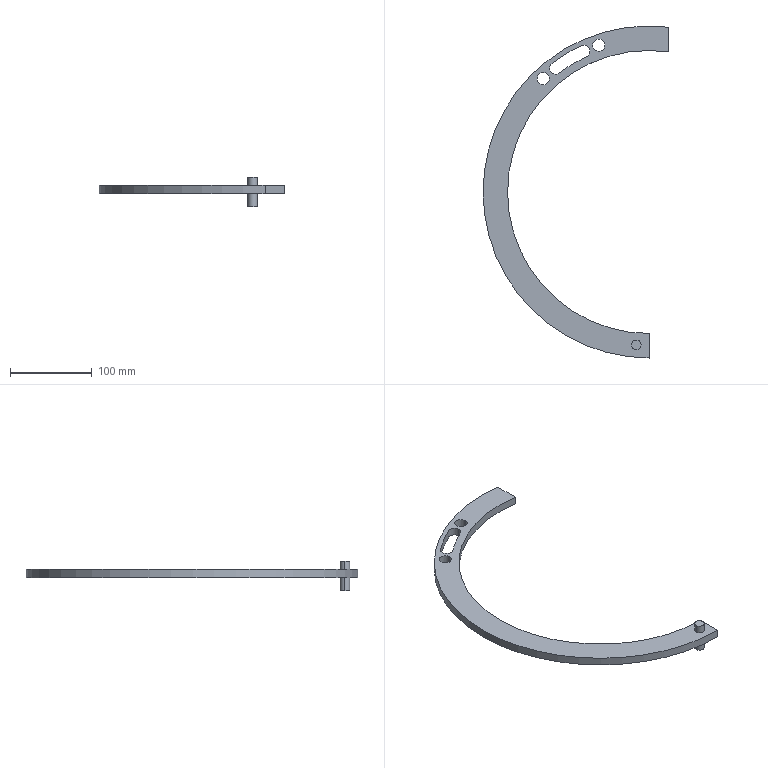Part | SolidWorks | features Cut 1, Extrusion 1, ICE 1 | 1 solid | 21 faces | box 227.579 x 406.59 x 36 mm | volume 176233 mm3 | cylinder 15 | plane 6 | commonest cylinder face diameters 15 x7 11.641 x4 346.59 x1 365 x1 395 x1 406.59 x1
STEP:
#1=CARTESIAN_POINT('',(-413.724,321.633,-10.));
#2=VERTEX_POINT('',#1);
#3=CARTESIAN_POINT('',(-428.724,321.633,-10.));
#4=VERTEX_POINT('',#3);
#5=CARTESIAN_POINT('',(-421.224,321.633,-10.));
#6=DIRECTION('',(0.,0.,-1.));
#7=DIRECTION('',(-1.,0.,0.));
#8=AXIS2_PLACEMENT_3D('',#5,#6,#7);
#9=CIRCLE('',#8,7.5);
#10=EDGE_CURVE('',#2,#4,#9,.T.);
#11=ORIENTED_EDGE('',*,*,#10,.T.);
#12=CARTESIAN_POINT('',(-428.724,321.633,0.));
#13=VERTEX_POINT('',#12);
#14=CARTESIAN_POINT('',(-428.724,321.633,-26.));
#15=DIRECTION('',(0.,0.,1.));
#16=VECTOR('',#15,1000.);
#17=LINE('',#14,#16);
#18=EDGE_CURVE('',#4,#13,#17,.T.);
#19=ORIENTED_EDGE('',*,*,#18,.T.);
#20=CARTESIAN_POINT('',(-413.724,321.633,0.));
#21=VERTEX_POINT('',#20);
#22=CARTESIAN_POINT('',(-421.224,321.633,0.));
#23=DIRECTION('',(0.,0.,-1.));
#24=DIRECTION('',(-1.,0.,0.));
#25=AXIS2_PLACEMENT_3D('',#22,#23,#24);
#26=CIRCLE('',#25,7.5);
#27=EDGE_CURVE('',#21,#13,#26,.T.);
#28=ORIENTED_EDGE('',*,*,#27,.F.);
#29=CARTESIAN_POINT('',(-413.724,321.633,-26.));
#30=DIRECTION('',(0.,0.,1.));
#31=VECTOR('',#30,1000.);
#32=LINE('',#29,#31);
#33=EDGE_CURVE('',#2,#21,#32,.T.);
#34=ORIENTED_EDGE('',*,*,#33,.F.);
#35=EDGE_LOOP('',(#11,#19,#28,#34));
#36=FACE_OUTER_BOUND('',#35,.T.);
#37=CARTESIAN_POINT('',(-421.224,321.633,-26.));
#38=DIRECTION('',(0.,0.,1.));
#39=DIRECTION('',(1.,0.,0.));
#40=AXIS2_PLACEMENT_3D('',#37,#38,#39);
#41=CYLINDRICAL_SURFACE('',#40,7.5);
#42=ADVANCED_FACE('',(#36),#41,.F.);
#43=CARTESIAN_POINT('',(-345.629,362.487,-10.));
#44=VERTEX_POINT('',#43);
#45=CARTESIAN_POINT('',(-360.629,362.487,-10.));
#46=VERTEX_POINT('',#45);
#47=CARTESIAN_POINT('',(-353.129,362.487,-10.));
#48=DIRECTION('',(0.,0.,-1.));
#49=DIRECTION('',(-1.,0.,0.));
#50=AXIS2_PLACEMENT_3D('',#47,#48,#49);
#51=CIRCLE('',#50,7.5);
#52=EDGE_CURVE('',#44,#46,#51,.T.);
#53=ORIENTED_EDGE('',*,*,#52,.T.);
#54=CARTESIAN_POINT('',(-360.629,362.487,0.));
#55=VERTEX_POINT('',#54);
#56=CARTESIAN_POINT('',(-360.629,362.487,-26.));
#57=DIRECTION('',(0.,0.,1.));
#58=VECTOR('',#57,1000.);
#59=LINE('',#56,#58);
#60=EDGE_CURVE('',#46,#55,#59,.T.);
#61=ORIENTED_EDGE('',*,*,#60,.T.);
#62=CARTESIAN_POINT('',(-345.629,362.487,0.));
#63=VERTEX_POINT('',#62);
#64=CARTESIAN_POINT('',(-353.129,362.487,0.));
#65=DIRECTION('',(0.,0.,-1.));
#66=DIRECTION('',(-1.,0.,0.));
#67=AXIS2_PLACEMENT_3D('',#64,#65,#66);
#68=CIRCLE('',#67,7.5);
#69=EDGE_CURVE('',#63,#55,#68,.T.);
#70=ORIENTED_EDGE('',*,*,#69,.F.);
#71=CARTESIAN_POINT('',(-345.629,362.487,-26.));
#72=DIRECTION('',(0.,0.,1.));
#73=VECTOR('',#72,1000.);
#74=LINE('',#71,#73);
#75=EDGE_CURVE('',#44,#63,#74,.T.);
#76=ORIENTED_EDGE('',*,*,#75,.F.);
#77=EDGE_LOOP('',(#53,#61,#70,#76));
#78=FACE_OUTER_BOUND('',#77,.T.);
#79=CARTESIAN_POINT('',(-353.129,362.487,-26.));
#80=DIRECTION('',(0.,0.,1.));
#81=DIRECTION('',(1.,0.,0.));
#82=AXIS2_PLACEMENT_3D('',#79,#80,#81);
#83=CYLINDRICAL_SURFACE('',#82,7.5);
#84=ADVANCED_FACE('',(#78),#83,.F.);
#85=CARTESIAN_POINT('',(-374.845,361.823,-10.));
#86=VERTEX_POINT('',#85);
#87=CARTESIAN_POINT('',(-364.183,355.022,-10.));
#88=VERTEX_POINT('',#87);
#89=CARTESIAN_POINT('',(-371.683,355.022,-10.));
#90=DIRECTION('',(0.,0.,-1.));
#91=DIRECTION('',(-1.,0.,0.));
#92=AXIS2_PLACEMENT_3D('',#89,#90,#91);
#93=CIRCLE('',#92,7.5);
#94=EDGE_CURVE('',#86,#88,#93,.T.);
#95=ORIENTED_EDGE('',*,*,#94,.T.);
#96=CARTESIAN_POINT('',(-364.183,355.022,0.));
#97=VERTEX_POINT('',#96);
#98=CARTESIAN_POINT('',(-364.183,355.022,-26.));
#99=DIRECTION('',(0.,0.,1.));
#100=VECTOR('',#99,1000.);
#101=LINE('',#98,#100);
#102=EDGE_CURVE('',#88,#97,#101,.T.);
#103=ORIENTED_EDGE('',*,*,#102,.T.);
#104=CARTESIAN_POINT('',(-374.845,361.823,0.));
#105=VERTEX_POINT('',#104);
#106=CARTESIAN_POINT('',(-371.683,355.022,0.));
#107=DIRECTION('',(0.,0.,-1.));
#108=DIRECTION('',(-1.,0.,0.));
#109=AXIS2_PLACEMENT_3D('',#106,#107,#108);
#110=CIRCLE('',#109,7.5);
#111=EDGE_CURVE('',#105,#97,#110,.T.);
#112=ORIENTED_EDGE('',*,*,#111,.F.);
#113=CARTESIAN_POINT('',(-374.845,361.823,-26.));
#114=DIRECTION('',(0.,0.,1.));
#115=VECTOR('',#114,1000.);
#116=LINE('',#113,#115);
#117=EDGE_CURVE('',#86,#105,#116,.T.);
#118=ORIENTED_EDGE('',*,*,#117,.F.);
#119=EDGE_LOOP('',(#95,#103,#112,#118));
#120=FACE_OUTER_BOUND('',#119,.T.);
#121=CARTESIAN_POINT('',(-371.683,355.022,-26.));
#122=DIRECTION('',(0.,0.,1.));
#123=DIRECTION('',(1.,0.,0.));
#124=AXIS2_PLACEMENT_3D('',#121,#122,#123);
#125=CYLINDRICAL_SURFACE('',#124,7.5);
#126=ADVANCED_FACE('',(#120),#125,.F.);
#127=CARTESIAN_POINT('',(-301.381,-4.52,-26.));
#128=VERTEX_POINT('',#127);
#129=CARTESIAN_POINT('',(-313.022,-4.52,-26.));
#130=VERTEX_POINT('',#129);
#131=CARTESIAN_POINT('',(-307.202,-4.52,-26.));
#132=DIRECTION('',(0.,0.,1.));
#133=DIRECTION('',(1.,0.,0.));
#134=AXIS2_PLACEMENT_3D('',#131,#132,#133);
#135=CIRCLE('',#134,5.82);
#136=EDGE_CURVE('',#128,#130,#135,.T.);
#137=ORIENTED_EDGE('',*,*,#136,.T.);
#138=CARTESIAN_POINT('',(-313.022,-4.52,-10.));
#139=VERTEX_POINT('',#138);
#140=CARTESIAN_POINT('',(-313.022,-4.52,-26.));
#141=DIRECTION('',(0.,0.,1.));
#142=VECTOR('',#141,1000.);
#143=LINE('',#140,#142);
#144=EDGE_CURVE('',#130,#139,#143,.T.);
#145=ORIENTED_EDGE('',*,*,#144,.T.);
#146=CARTESIAN_POINT('',(-301.381,-4.52,-10.));
#147=VERTEX_POINT('',#146);
#148=CARTESIAN_POINT('',(-307.202,-4.52,-10.));
#149=DIRECTION('',(0.,0.,-1.));
#150=DIRECTION('',(-1.,0.,0.));
#151=AXIS2_PLACEMENT_3D('',#148,#149,#150);
#152=CIRCLE('',#151,5.82);
#153=EDGE_CURVE('',#139,#147,#152,.T.);
#154=ORIENTED_EDGE('',*,*,#153,.T.);
#155=CARTESIAN_POINT('',(-301.381,-4.52,-26.));
#156=DIRECTION('',(0.,0.,1.));
#157=VECTOR('',#156,1000.);
#158=LINE('',#155,#157);
#159=EDGE_CURVE('',#128,#147,#158,.T.);
#160=ORIENTED_EDGE('',*,*,#159,.F.);
#161=EDGE_LOOP('',(#137,#145,#154,#160));
#162=FACE_OUTER_BOUND('',#161,.T.);
#163=CARTESIAN_POINT('',(-307.202,-4.52,-26.));
#164=DIRECTION('',(0.,0.,1.));
#165=DIRECTION('',(1.,0.,0.));
#166=AXIS2_PLACEMENT_3D('',#163,#164,#165);
#167=CYLINDRICAL_SURFACE('',#166,5.82);
#168=ADVANCED_FACE('',(#162),#167,.T.);
#169=CARTESIAN_POINT('',(-313.022,-4.52,0.));
#170=VERTEX_POINT('',#169);
#171=CARTESIAN_POINT('',(-301.381,-4.52,0.));
#172=VERTEX_POINT('',#171);
#173=CARTESIAN_POINT('',(-307.202,-4.52,0.));
#174=DIRECTION('',(0.,0.,-1.));
#175=DIRECTION('',(-1.,0.,0.));
#176=AXIS2_PLACEMENT_3D('',#173,#174,#175);
#177=CIRCLE('',#176,5.82);
#178=EDGE_CURVE('',#170,#172,#177,.T.);
#179=ORIENTED_EDGE('',*,*,#178,.F.);
#180=CARTESIAN_POINT('',(-313.022,-4.52,10.));
#181=VERTEX_POINT('',#180);
#182=CARTESIAN_POINT('',(-313.022,-4.52,-26.));
#183=DIRECTION('',(0.,0.,1.));
#184=VECTOR('',#183,1000.);
#185=LINE('',#182,#184);
#186=EDGE_CURVE('',#170,#181,#185,.T.);
#187=ORIENTED_EDGE('',*,*,#186,.T.);
#188=CARTESIAN_POINT('',(-301.381,-4.52,10.));
#189=VERTEX_POINT('',#188);
#190=CARTESIAN_POINT('',(-307.202,-4.52,10.));
#191=DIRECTION('',(0.,0.,1.));
#192=DIRECTION('',(1.,0.,0.));
#193=AXIS2_PLACEMENT_3D('',#190,#191,#192);
#194=CIRCLE('',#193,5.82);
#195=EDGE_CURVE('',#189,#181,#194,.T.);
#196=ORIENTED_EDGE('',*,*,#195,.F.);
#197=CARTESIAN_POINT('',(-301.381,-4.52,-26.));
#198=DIRECTION('',(0.,0.,1.));
#199=VECTOR('',#198,1000.);
#200=LINE('',#197,#199);
#201=EDGE_CURVE('',#172,#189,#200,.T.);
#202=ORIENTED_EDGE('',*,*,#201,.F.);
#203=EDGE_LOOP('',(#179,#187,#196,#202));
#204=FACE_OUTER_BOUND('',#203,.T.);
#205=CARTESIAN_POINT('',(-307.202,-4.52,-26.));
#206=DIRECTION('',(0.,0.,1.));
#207=DIRECTION('',(1.,0.,0.));
#208=AXIS2_PLACEMENT_3D('',#205,#206,#207);
#209=CYLINDRICAL_SURFACE('',#208,5.82);
#210=ADVANCED_FACE('',(#204),#209,.T.);
#211=ORIENTED_EDGE('',*,*,#10,.F.);
#212=CARTESIAN_POINT('',(-421.224,321.633,-10.));
#213=DIRECTION('',(0.,0.,-1.));
#214=DIRECTION('',(-1.,0.,0.));
#215=AXIS2_PLACEMENT_3D('',#212,#213,#214);
#216=CIRCLE('',#215,7.5);
#217=EDGE_CURVE('',#4,#2,#216,.T.);
#218=ORIENTED_EDGE('',*,*,#217,.F.);
#219=EDGE_LOOP('',(#211,#218));
#220=FACE_BOUND('',#219,.T.);
#221=ORIENTED_EDGE('',*,*,#52,.F.);
#222=CARTESIAN_POINT('',(-353.129,362.487,-10.));
#223=DIRECTION('',(0.,0.,-1.));
#224=DIRECTION('',(-1.,0.,0.));
#225=AXIS2_PLACEMENT_3D('',#222,#223,#224);
#226=CIRCLE('',#225,7.5);
#227=EDGE_CURVE('',#46,#44,#226,.T.);
#228=ORIENTED_EDGE('',*,*,#227,.F.);
#229=EDGE_LOOP('',(#221,#228));
#230=FACE_BOUND('',#229,.T.);
#231=ORIENTED_EDGE('',*,*,#94,.F.);
#232=CARTESIAN_POINT('',(-410.433,340.469,-10.));
#233=VERTEX_POINT('',#232);
#234=CARTESIAN_POINT('',(-291.585,182.731,-10.));
#235=DIRECTION('',(0.,0.,-1.));
#236=DIRECTION('',(-1.,0.,0.));
#237=AXIS2_PLACEMENT_3D('',#234,#235,#236);
#238=CIRCLE('',#237,197.5);
#239=EDGE_CURVE('',#233,#86,#238,.T.);
#240=ORIENTED_EDGE('',*,*,#239,.F.);
#241=CARTESIAN_POINT('',(-401.406,328.489,-10.));
#242=VERTEX_POINT('',#241);
#243=CARTESIAN_POINT('',(-405.919,334.479,-10.));
#244=DIRECTION('',(0.,0.,-1.));
#245=DIRECTION('',(-1.,0.,0.));
#246=AXIS2_PLACEMENT_3D('',#243,#244,#245);
#247=CIRCLE('',#246,7.5);
#248=EDGE_CURVE('',#242,#233,#247,.T.);
#249=ORIENTED_EDGE('',*,*,#248,.F.);
#250=CARTESIAN_POINT('',(-368.522,348.221,-10.));
#251=VERTEX_POINT('',#250);
#252=CARTESIAN_POINT('',(-291.585,182.731,-10.));
#253=DIRECTION('',(0.,0.,1.));
#254=DIRECTION('',(-1.,0.,0.));
#255=AXIS2_PLACEMENT_3D('',#252,#253,#254);
#256=CIRCLE('',#255,182.5);
#257=EDGE_CURVE('',#251,#242,#256,.T.);
#258=ORIENTED_EDGE('',*,*,#257,.F.);
#259=CARTESIAN_POINT('',(-371.683,355.022,-10.));
#260=DIRECTION('',(0.,0.,-1.));
#261=DIRECTION('',(-1.,0.,0.));
#262=AXIS2_PLACEMENT_3D('',#259,#260,#261);
#263=CIRCLE('',#262,7.5);
#264=EDGE_CURVE('',#88,#251,#263,.T.);
#265=ORIENTED_EDGE('',*,*,#264,.F.);
#266=EDGE_LOOP('',(#231,#240,#249,#258,#265));
#267=FACE_BOUND('',#266,.T.);
#268=CARTESIAN_POINT('',(-307.202,-4.52,-10.));
#269=DIRECTION('',(0.,0.,-1.));
#270=DIRECTION('',(-1.,0.,0.));
#271=AXIS2_PLACEMENT_3D('',#268,#269,#270);
#272=CIRCLE('',#271,5.82);
#273=EDGE_CURVE('',#147,#139,#272,.T.);
#274=ORIENTED_EDGE('',*,*,#273,.F.);
#275=ORIENTED_EDGE('',*,*,#153,.F.);
#276=EDGE_LOOP('',(#274,#275));
#277=FACE_BOUND('',#276,.T.);
#278=CARTESIAN_POINT('',(-291.585,9.436,-10.));
#279=VERTEX_POINT('',#278);
#280=CARTESIAN_POINT('',(-267.302,354.316,-10.));
#281=VERTEX_POINT('',#280);
#282=CARTESIAN_POINT('',(-291.585,182.731,-10.));
#283=DIRECTION('',(0.,0.,-1.));
#284=DIRECTION('',(-1.,0.,0.));
#285=AXIS2_PLACEMENT_3D('',#282,#283,#284);
#286=CIRCLE('',#285,173.295);
#287=EDGE_CURVE('',#279,#281,#286,.T.);
#288=ORIENTED_EDGE('',*,*,#287,.F.);
#289=CARTESIAN_POINT('',(-291.585,-20.564,-10.));
#290=VERTEX_POINT('',#289);
#291=CARTESIAN_POINT('',(-291.585,9.436,-10.));
#292=DIRECTION('',(0.,1.,0.));
#293=VECTOR('',#292,1000.);
#294=LINE('',#291,#293);
#295=EDGE_CURVE('',#290,#279,#294,.T.);
#296=ORIENTED_EDGE('',*,*,#295,.F.);
#297=CARTESIAN_POINT('',(-267.317,384.572,-10.));
#298=VERTEX_POINT('',#297);
#299=CARTESIAN_POINT('',(-291.585,182.731,-10.));
#300=DIRECTION('',(0.,0.,1.));
#301=DIRECTION('',(-1.,0.,0.));
#302=AXIS2_PLACEMENT_3D('',#299,#300,#301);
#303=CIRCLE('',#302,203.295);
#304=EDGE_CURVE('',#298,#290,#303,.T.);
#305=ORIENTED_EDGE('',*,*,#304,.F.);
#306=CARTESIAN_POINT('',(-267.317,384.572,-10.));
#307=DIRECTION('',(-0.0005094,1.,0.));
#308=VECTOR('',#307,1000.);
#309=LINE('',#306,#308);
#310=EDGE_CURVE('',#281,#298,#309,.T.);
#311=ORIENTED_EDGE('',*,*,#310,.F.);
#312=EDGE_LOOP('',(#288,#296,#305,#311));
#313=FACE_OUTER_BOUND('',#312,.T.);
#314=CARTESIAN_POINT('',(-291.585,182.731,-10.));
#315=DIRECTION('',(0.,0.,-1.));
#316=DIRECTION('',(-1.,0.,0.));
#317=AXIS2_PLACEMENT_3D('',#314,#315,#316);
#318=PLANE('',#317);
#319=ADVANCED_FACE('',(#220,#230,#267,#277,#313),#318,.T.);
#320=ORIENTED_EDGE('',*,*,#27,.T.);
#321=CARTESIAN_POINT('',(-421.224,321.633,0.));
#322=DIRECTION('',(0.,0.,-1.));
#323=DIRECTION('',(-1.,0.,0.));
#324=AXIS2_PLACEMENT_3D('',#321,#322,#323);
#325=CIRCLE('',#324,7.5);
#326=EDGE_CURVE('',#13,#21,#325,.T.);
#327=ORIENTED_EDGE('',*,*,#326,.T.);
#328=EDGE_LOOP('',(#320,#327));
#329=FACE_BOUND('',#328,.T.);
#330=ORIENTED_EDGE('',*,*,#69,.T.);
#331=CARTESIAN_POINT('',(-353.129,362.487,0.));
#332=DIRECTION('',(0.,0.,-1.));
#333=DIRECTION('',(-1.,0.,0.));
#334=AXIS2_PLACEMENT_3D('',#331,#332,#333);
#335=CIRCLE('',#334,7.5);
#336=EDGE_CURVE('',#55,#63,#335,.T.);
#337=ORIENTED_EDGE('',*,*,#336,.T.);
#338=EDGE_LOOP('',(#330,#337));
#339=FACE_BOUND('',#338,.T.);
#340=CARTESIAN_POINT('',(-410.433,340.469,0.));
#341=VERTEX_POINT('',#340);
#342=CARTESIAN_POINT('',(-291.585,182.731,0.));
#343=DIRECTION('',(0.,0.,-1.));
#344=DIRECTION('',(-1.,0.,0.));
#345=AXIS2_PLACEMENT_3D('',#342,#343,#344);
#346=CIRCLE('',#345,197.5);
#347=EDGE_CURVE('',#341,#105,#346,.T.);
#348=ORIENTED_EDGE('',*,*,#347,.T.);
#349=ORIENTED_EDGE('',*,*,#111,.T.);
#350=CARTESIAN_POINT('',(-368.522,348.221,0.));
#351=VERTEX_POINT('',#350);
#352=CARTESIAN_POINT('',(-371.683,355.022,0.));
#353=DIRECTION('',(0.,0.,-1.));
#354=DIRECTION('',(-1.,0.,0.));
#355=AXIS2_PLACEMENT_3D('',#352,#353,#354);
#356=CIRCLE('',#355,7.5);
#357=EDGE_CURVE('',#97,#351,#356,.T.);
#358=ORIENTED_EDGE('',*,*,#357,.T.);
#359=CARTESIAN_POINT('',(-401.406,328.489,0.));
#360=VERTEX_POINT('',#359);
#361=CARTESIAN_POINT('',(-291.585,182.731,0.));
#362=DIRECTION('',(0.,0.,1.));
#363=DIRECTION('',(-1.,0.,0.));
#364=AXIS2_PLACEMENT_3D('',#361,#362,#363);
#365=CIRCLE('',#364,182.5);
#366=EDGE_CURVE('',#351,#360,#365,.T.);
#367=ORIENTED_EDGE('',*,*,#366,.T.);
#368=CARTESIAN_POINT('',(-405.919,334.479,0.));
#369=DIRECTION('',(0.,0.,-1.));
#370=DIRECTION('',(-1.,0.,0.));
#371=AXIS2_PLACEMENT_3D('',#368,#369,#370);
#372=CIRCLE('',#371,7.5);
#373=EDGE_CURVE('',#360,#341,#372,.T.);
#374=ORIENTED_EDGE('',*,*,#373,.T.);
#375=EDGE_LOOP('',(#348,#349,#358,#367,#374));
#376=FACE_BOUND('',#375,.T.);
#377=CARTESIAN_POINT('',(-307.202,-4.52,0.));
#378=DIRECTION('',(0.,0.,-1.));
#379=DIRECTION('',(-1.,0.,0.));
#380=AXIS2_PLACEMENT_3D('',#377,#378,#379);
#381=CIRCLE('',#380,5.82);
#382=EDGE_CURVE('',#172,#170,#381,.T.);
#383=ORIENTED_EDGE('',*,*,#382,.T.);
#384=ORIENTED_EDGE('',*,*,#178,.T.);
#385=EDGE_LOOP('',(#383,#384));
#386=FACE_BOUND('',#385,.T.);
#387=CARTESIAN_POINT('',(-291.585,9.436,0.));
#388=VERTEX_POINT('',#387);
#389=CARTESIAN_POINT('',(-267.302,354.316,0.));
#390=VERTEX_POINT('',#389);
#391=CARTESIAN_POINT('',(-291.585,182.731,0.));
#392=DIRECTION('',(0.,0.,-1.));
#393=DIRECTION('',(-1.,0.,0.));
#394=AXIS2_PLACEMENT_3D('',#391,#392,#393);
#395=CIRCLE('',#394,173.295);
#396=EDGE_CURVE('',#388,#390,#395,.T.);
#397=ORIENTED_EDGE('',*,*,#396,.T.);
#398=CARTESIAN_POINT('',(-267.317,384.572,0.));
#399=VERTEX_POINT('',#398);
#400=CARTESIAN_POINT('',(-267.317,384.572,0.));
#401=DIRECTION('',(-0.0005094,1.,0.));
#402=VECTOR('',#401,1000.);
#403=LINE('',#400,#402);
#404=EDGE_CURVE('',#390,#399,#403,.T.);
#405=ORIENTED_EDGE('',*,*,#404,.T.);
#406=CARTESIAN_POINT('',(-291.585,-20.564,0.));
#407=VERTEX_POINT('',#406);
#408=CARTESIAN_POINT('',(-291.585,182.731,0.));
#409=DIRECTION('',(0.,0.,1.));
#410=DIRECTION('',(1.,0.,0.));
#411=AXIS2_PLACEMENT_3D('',#408,#409,#410);
#412=CIRCLE('',#411,203.295);
#413=EDGE_CURVE('',#399,#407,#412,.T.);
#414=ORIENTED_EDGE('',*,*,#413,.T.);
#415=CARTESIAN_POINT('',(-291.585,9.436,0.));
#416=DIRECTION('',(0.,1.,0.));
#417=VECTOR('',#416,1000.);
#418=LINE('',#415,#417);
#419=EDGE_CURVE('',#407,#388,#418,.T.);
#420=ORIENTED_EDGE('',*,*,#419,.T.);
#421=EDGE_LOOP('',(#397,#405,#414,#420));
#422=FACE_OUTER_BOUND('',#421,.T.);
#423=CARTESIAN_POINT('',(-291.585,182.731,0.));
#424=DIRECTION('',(0.,0.,-1.));
#425=DIRECTION('',(-1.,0.,0.));
#426=AXIS2_PLACEMENT_3D('',#423,#424,#425);
#427=PLANE('',#426);
#428=ADVANCED_FACE('',(#329,#339,#376,#386,#422),#427,.F.);
#429=CARTESIAN_POINT('',(-267.302,354.316,-475.948));
#430=DIRECTION('',(0.,0.,1.));
#431=VECTOR('',#430,1000.);
#432=LINE('',#429,#431);
#433=EDGE_CURVE('',#281,#390,#432,.T.);
#434=ORIENTED_EDGE('',*,*,#433,.F.);
#435=ORIENTED_EDGE('',*,*,#310,.T.);
#436=CARTESIAN_POINT('',(-267.317,384.572,-475.948));
#437=DIRECTION('',(0.,0.,1.));
#438=VECTOR('',#437,1000.);
#439=LINE('',#436,#438);
#440=EDGE_CURVE('',#298,#399,#439,.T.);
#441=ORIENTED_EDGE('',*,*,#440,.T.);
#442=ORIENTED_EDGE('',*,*,#404,.F.);
#443=EDGE_LOOP('',(#434,#435,#441,#442));
#444=FACE_OUTER_BOUND('',#443,.T.);
#445=CARTESIAN_POINT('',(-267.317,384.572,-475.948));
#446=DIRECTION('',(1.,0.0005094,0.));
#447=DIRECTION('',(-0.0005094,1.,0.));
#448=AXIS2_PLACEMENT_3D('',#445,#446,#447);
#449=PLANE('',#448);
#450=ADVANCED_FACE('',(#444),#449,.T.);
#451=ORIENTED_EDGE('',*,*,#440,.F.);
#452=ORIENTED_EDGE('',*,*,#304,.T.);
#453=CARTESIAN_POINT('',(-291.585,-20.564,-475.948));
#454=DIRECTION('',(0.,0.,1.));
#455=VECTOR('',#454,1000.);
#456=LINE('',#453,#455);
#457=EDGE_CURVE('',#290,#407,#456,.T.);
#458=ORIENTED_EDGE('',*,*,#457,.T.);
#459=ORIENTED_EDGE('',*,*,#413,.F.);
#460=EDGE_LOOP('',(#451,#452,#458,#459));
#461=FACE_OUTER_BOUND('',#460,.T.);
#462=CARTESIAN_POINT('',(-291.585,182.731,-475.948));
#463=DIRECTION('',(0.,0.,1.));
#464=DIRECTION('',(1.,0.,0.));
#465=AXIS2_PLACEMENT_3D('',#462,#463,#464);
#466=CYLINDRICAL_SURFACE('',#465,203.295);
#467=ADVANCED_FACE('',(#461),#466,.T.);
#468=ORIENTED_EDGE('',*,*,#457,.F.);
#469=ORIENTED_EDGE('',*,*,#295,.T.);
#470=CARTESIAN_POINT('',(-291.585,9.436,-475.948));
#471=DIRECTION('',(0.,0.,1.));
#472=VECTOR('',#471,1000.);
#473=LINE('',#470,#472);
#474=EDGE_CURVE('',#279,#388,#473,.T.);
#475=ORIENTED_EDGE('',*,*,#474,.T.);
#476=ORIENTED_EDGE('',*,*,#419,.F.);
#477=EDGE_LOOP('',(#468,#469,#475,#476));
#478=FACE_OUTER_BOUND('',#477,.T.);
#479=CARTESIAN_POINT('',(-291.585,9.436,-475.948));
#480=DIRECTION('',(1.,0.,0.));
#481=DIRECTION('',(0.,1.,0.));
#482=AXIS2_PLACEMENT_3D('',#479,#480,#481);
#483=PLANE('',#482);
#484=ADVANCED_FACE('',(#478),#483,.T.);
#485=ORIENTED_EDGE('',*,*,#474,.F.);
#486=ORIENTED_EDGE('',*,*,#287,.T.);
#487=ORIENTED_EDGE('',*,*,#433,.T.);
#488=ORIENTED_EDGE('',*,*,#396,.F.);
#489=EDGE_LOOP('',(#485,#486,#487,#488));
#490=FACE_OUTER_BOUND('',#489,.T.);
#491=CARTESIAN_POINT('',(-291.585,182.731,-475.948));
#492=DIRECTION('',(0.,0.,1.));
#493=DIRECTION('',(1.,0.,0.));
#494=AXIS2_PLACEMENT_3D('',#491,#492,#493);
#495=CYLINDRICAL_SURFACE('',#494,173.295);
#496=ADVANCED_FACE('',(#490),#495,.F.);
#497=ORIENTED_EDGE('',*,*,#195,.T.);
#498=CARTESIAN_POINT('',(-307.202,-4.52,10.));
#499=DIRECTION('',(0.,0.,1.));
#500=DIRECTION('',(1.,0.,0.));
#501=AXIS2_PLACEMENT_3D('',#498,#499,#500);
#502=CIRCLE('',#501,5.82);
#503=EDGE_CURVE('',#181,#189,#502,.T.);
#504=ORIENTED_EDGE('',*,*,#503,.T.);
#505=EDGE_LOOP('',(#497,#504));
#506=FACE_OUTER_BOUND('',#505,.T.);
#507=CARTESIAN_POINT('',(-307.202,-4.52,10.));
#508=DIRECTION('',(0.,0.,1.));
#509=DIRECTION('',(1.,0.,0.));
#510=AXIS2_PLACEMENT_3D('',#507,#508,#509);
#511=PLANE('',#510);
#512=ADVANCED_FACE('',(#506),#511,.T.);
#513=ORIENTED_EDGE('',*,*,#186,.F.);
#514=ORIENTED_EDGE('',*,*,#382,.F.);
#515=ORIENTED_EDGE('',*,*,#201,.T.);
#516=ORIENTED_EDGE('',*,*,#503,.F.);
#517=EDGE_LOOP('',(#513,#514,#515,#516));
#518=FACE_OUTER_BOUND('',#517,.T.);
#519=CARTESIAN_POINT('',(-307.202,-4.52,-26.));
#520=DIRECTION('',(0.,0.,1.));
#521=DIRECTION('',(1.,0.,0.));
#522=AXIS2_PLACEMENT_3D('',#519,#520,#521);
#523=CYLINDRICAL_SURFACE('',#522,5.82);
#524=ADVANCED_FACE('',(#518),#523,.T.);
#525=ORIENTED_EDGE('',*,*,#144,.F.);
#526=CARTESIAN_POINT('',(-307.202,-4.52,-26.));
#527=DIRECTION('',(0.,0.,1.));
#528=DIRECTION('',(1.,0.,0.));
#529=AXIS2_PLACEMENT_3D('',#526,#527,#528);
#530=CIRCLE('',#529,5.82);
#531=EDGE_CURVE('',#130,#128,#530,.T.);
#532=ORIENTED_EDGE('',*,*,#531,.T.);
#533=ORIENTED_EDGE('',*,*,#159,.T.);
#534=ORIENTED_EDGE('',*,*,#273,.T.);
#535=EDGE_LOOP('',(#525,#532,#533,#534));
#536=FACE_OUTER_BOUND('',#535,.T.);
#537=CARTESIAN_POINT('',(-307.202,-4.52,-26.));
#538=DIRECTION('',(0.,0.,1.));
#539=DIRECTION('',(1.,0.,0.));
#540=AXIS2_PLACEMENT_3D('',#537,#538,#539);
#541=CYLINDRICAL_SURFACE('',#540,5.82);
#542=ADVANCED_FACE('',(#536),#541,.T.);
#543=ORIENTED_EDGE('',*,*,#136,.F.);
#544=ORIENTED_EDGE('',*,*,#531,.F.);
#545=EDGE_LOOP('',(#543,#544));
#546=FACE_OUTER_BOUND('',#545,.T.);
#547=CARTESIAN_POINT('',(-307.202,-4.52,-26.));
#548=DIRECTION('',(0.,0.,1.));
#549=DIRECTION('',(1.,0.,0.));
#550=AXIS2_PLACEMENT_3D('',#547,#548,#549);
#551=PLANE('',#550);
#552=ADVANCED_FACE('',(#546),#551,.F.);
#553=ORIENTED_EDGE('',*,*,#102,.F.);
#554=ORIENTED_EDGE('',*,*,#264,.T.);
#555=CARTESIAN_POINT('',(-368.522,348.221,-26.));
#556=DIRECTION('',(0.,0.,1.));
#557=VECTOR('',#556,1000.);
#558=LINE('',#555,#557);
#559=EDGE_CURVE('',#251,#351,#558,.T.);
#560=ORIENTED_EDGE('',*,*,#559,.T.);
#561=ORIENTED_EDGE('',*,*,#357,.F.);
#562=EDGE_LOOP('',(#553,#554,#560,#561));
#563=FACE_OUTER_BOUND('',#562,.T.);
#564=CARTESIAN_POINT('',(-371.683,355.022,-26.));
#565=DIRECTION('',(0.,0.,1.));
#566=DIRECTION('',(1.,0.,0.));
#567=AXIS2_PLACEMENT_3D('',#564,#565,#566);
#568=CYLINDRICAL_SURFACE('',#567,7.5);
#569=ADVANCED_FACE('',(#563),#568,.F.);
#570=ORIENTED_EDGE('',*,*,#257,.T.);
#571=CARTESIAN_POINT('',(-401.406,328.489,-26.));
#572=DIRECTION('',(0.,0.,1.));
#573=VECTOR('',#572,1000.);
#574=LINE('',#571,#573);
#575=EDGE_CURVE('',#242,#360,#574,.T.);
#576=ORIENTED_EDGE('',*,*,#575,.T.);
#577=ORIENTED_EDGE('',*,*,#366,.F.);
#578=ORIENTED_EDGE('',*,*,#559,.F.);
#579=EDGE_LOOP('',(#570,#576,#577,#578));
#580=FACE_OUTER_BOUND('',#579,.T.);
#581=CARTESIAN_POINT('',(-291.585,182.731,-26.));
#582=DIRECTION('',(0.,0.,1.));
#583=DIRECTION('',(1.,0.,0.));
#584=AXIS2_PLACEMENT_3D('',#581,#582,#583);
#585=CYLINDRICAL_SURFACE('',#584,182.5);
#586=ADVANCED_FACE('',(#580),#585,.T.);
#587=ORIENTED_EDGE('',*,*,#248,.T.);
#588=CARTESIAN_POINT('',(-410.433,340.469,-26.));
#589=DIRECTION('',(0.,0.,1.));
#590=VECTOR('',#589,1000.);
#591=LINE('',#588,#590);
#592=EDGE_CURVE('',#233,#341,#591,.T.);
#593=ORIENTED_EDGE('',*,*,#592,.T.);
#594=ORIENTED_EDGE('',*,*,#373,.F.);
#595=ORIENTED_EDGE('',*,*,#575,.F.);
#596=EDGE_LOOP('',(#587,#593,#594,#595));
#597=FACE_OUTER_BOUND('',#596,.T.);
#598=CARTESIAN_POINT('',(-405.919,334.479,-26.));
#599=DIRECTION('',(0.,0.,1.));
#600=DIRECTION('',(1.,0.,0.));
#601=AXIS2_PLACEMENT_3D('',#598,#599,#600);
#602=CYLINDRICAL_SURFACE('',#601,7.5);
#603=ADVANCED_FACE('',(#597),#602,.F.);
#604=ORIENTED_EDGE('',*,*,#239,.T.);
#605=ORIENTED_EDGE('',*,*,#117,.T.);
#606=ORIENTED_EDGE('',*,*,#347,.F.);
#607=ORIENTED_EDGE('',*,*,#592,.F.);
#608=EDGE_LOOP('',(#604,#605,#606,#607));
#609=FACE_OUTER_BOUND('',#608,.T.);
#610=CARTESIAN_POINT('',(-291.585,182.731,-26.));
#611=DIRECTION('',(0.,0.,1.));
#612=DIRECTION('',(1.,0.,0.));
#613=AXIS2_PLACEMENT_3D('',#610,#611,#612);
#614=CYLINDRICAL_SURFACE('',#613,197.5);
#615=ADVANCED_FACE('',(#609),#614,.F.);
#616=ORIENTED_EDGE('',*,*,#60,.F.);
#617=ORIENTED_EDGE('',*,*,#227,.T.);
#618=ORIENTED_EDGE('',*,*,#75,.T.);
#619=ORIENTED_EDGE('',*,*,#336,.F.);
#620=EDGE_LOOP('',(#616,#617,#618,#619));
#621=FACE_OUTER_BOUND('',#620,.T.);
#622=CARTESIAN_POINT('',(-353.129,362.487,-26.));
#623=DIRECTION('',(0.,0.,1.));
#624=DIRECTION('',(1.,0.,0.));
#625=AXIS2_PLACEMENT_3D('',#622,#623,#624);
#626=CYLINDRICAL_SURFACE('',#625,7.5);
#627=ADVANCED_FACE('',(#621),#626,.F.);
#628=ORIENTED_EDGE('',*,*,#18,.F.);
#629=ORIENTED_EDGE('',*,*,#217,.T.);
#630=ORIENTED_EDGE('',*,*,#33,.T.);
#631=ORIENTED_EDGE('',*,*,#326,.F.);
#632=EDGE_LOOP('',(#628,#629,#630,#631));
#633=FACE_OUTER_BOUND('',#632,.T.);
#634=CARTESIAN_POINT('',(-421.224,321.633,-26.));
#635=DIRECTION('',(0.,0.,1.));
#636=DIRECTION('',(1.,0.,0.));
#637=AXIS2_PLACEMENT_3D('',#634,#635,#636);
#638=CYLINDRICAL_SURFACE('',#637,7.5);
#639=ADVANCED_FACE('',(#633),#638,.F.);
#640=CLOSED_SHELL('',(#42,#84,#126,#168,#210,#319,#428,#450,#467,#484,#496,#512,#524,#542,#552,#569,#586,#603,#615,#627,#639));
#641=MANIFOLD_SOLID_BREP('',#640);
#642=CARTESIAN_POINT('',(0.,0.,0.));
#643=DIRECTION('',(0.,0.,1.));
#644=DIRECTION('',(1.,0.,0.));
#645=AXIS2_PLACEMENT_3D('',#642,#643,#644);
#646=(LENGTH_UNIT()NAMED_UNIT(*)SI_UNIT(.MILLI.,.METRE.));
#647=UNCERTAINTY_MEASURE_WITH_UNIT(LENGTH_MEASURE(0.00001),#646,'','');
#648=(NAMED_UNIT(*)PLANE_ANGLE_UNIT()SI_UNIT($,.RADIAN.));
#649=(NAMED_UNIT(*)SI_UNIT($,.STERADIAN.)SOLID_ANGLE_UNIT());
#650=(GEOMETRIC_REPRESENTATION_CONTEXT(3)GLOBAL_UNCERTAINTY_ASSIGNED_CONTEXT((#647))GLOBAL_UNIT_ASSIGNED_CONTEXT((#646,#648,#649))REPRESENTATION_CONTEXT('',''));
#651=ADVANCED_BREP_SHAPE_REPRESENTATION('',(#641,#645),#650);